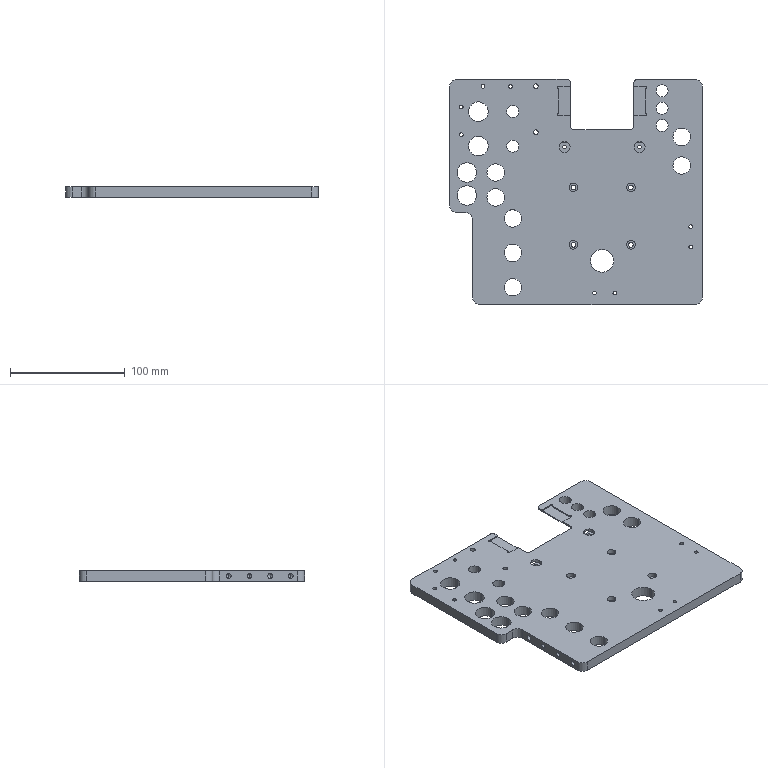NC program | NX | posted with a generic post | part box 220 x 196 x 9 mm
Lines 1 to 130 of 7489:
N10 G17 G21 G94 G90
(FLOOR_WALL_COPY , TOOL : D80)
N12 T19 M6
N14 G54
N16 G17 G0 G90 X-157. Y99.997 S6500 M3
N18 G43 Z30. H19
N20 Z3.
N22 G94 G1 Z0. F1500.
N24 X-152.
N26 X152.
N28 Y43.998
N30 X-152.
N32 Y-12.001
N34 X152.
N36 Y-68.
N38 X-152.
N40 X-157.
N42 Z3.
N44 G0 Z30.
N46 M5
(DRILLING_COPY_1 , TOOL : D6A45)
N48 T01 M6
N50 G54
N52 G17 G0 G90 X100. Y-48. S5000 M3
N54 G43 Z30. H1
N56 G94 G81 G98 Z-1. F350. R3.
N58 Y-30.2
N60 X92. Y23.
N62 Y48.
N64 X75. Y88.
N66 Y73.
N68 Y58.
N70 X55.35 Y39.2
N72 X47.75 Y4.
N74 Y-46.
N76 X33.863 Y-88.
N78 X16.063
N80 X22.74 Y-60.
N82 X-2.25 Y-46.
N84 Y4.
N86 X-9.95 Y39.2
N88 X-35. Y52.
N90 X-55. Y40.
N92 Y70.
N94 X-35. Y92.
N96 X-57.
N98 X-81.
N100 X-85. Y70.
N102 X-100. Y74.
N104 Y50.
N106 X-85. Y40.
N108 X-70. Y17.
N110 X-95.
N112 Y-3.
N114 X-70. Y-4.67
N116 X-55. Y-23.
N118 Y-53.
N120 Y-83.
N122 G80
N124 G0 X-55. Y-83. Z30.
N126 M5
(DRILLING_COPY_1_COPY_1_1_COPY_1 , TOOL : 3.3ZT)
N128 T03 M6
N130 G54
N132 G17 G0 G90 X-100. Y50. S2000 M3
N134 G43 Z30. H3
N136 G94 G83 G98 Z-11.491 F200. Q2. R3.
N138 Y74.
N140 X-81. Y92.
N142 X-57.
N144 X-9.95 Y39.2
N146 X55.35
N148 X100. Y-30.2
N150 Y-48.
N152 X33.863 Y-88.
N154 X16.063
N156 G80
N158 G0 X16.063 Y-88. Z30.
N160 M5
(DRILLING_COPY_1_COPY_1_1_COPY , TOOL : 4.2ZT)
N162 T04 M6
N164 G54
N166 G17 G0 G90 X-35. Y92. S2000 M3
N168 G43 Z30. H4
N170 G94 G83 G98 Z-7.762 F200. Q2. R3.
N172 Y52.
N174 X-2.25 Y4. Z-11.762
N176 X47.75
N178 Y-46.
N180 X-2.25
N182 G80
N184 G0 X-2.25 Y-46. Z30.
N186 M5
(DRILLING_COPY_1_COPY_1_1_COPY_COPY , TOOL : 10.5ZT)
N188 T16 M6
N190 G54
N192 G17 G0 G90 X-95. Y-3. S2000 M3
N194 G43 Z30. H16
N196 G94 G83 G98 Z-13.655 F200. Q2. R3.
N198 Y17.
N200 X-85. Y40.
N202 Y70.
N204 X-55.
N206 Y40.
N208 X-70. Y17.
N210 Y-4.67
N212 X-55. Y-23.
N214 Y-53.
N216 Y-83.
N218 X22.74 Y-60.
N220 X92. Y23.
N222 Y48.
N224 X75. Y58.
N226 Y73.
N228 Y88.
N230 G80
N232 G0 X75. Y88. Z30.
N234 M5